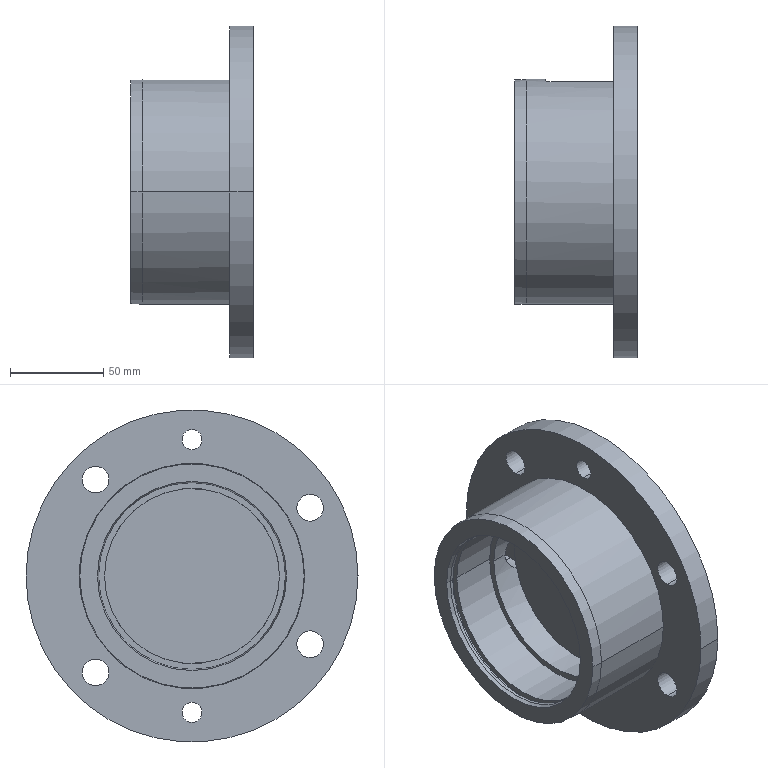Part | SolidWorks | features HoleWzd 2, ICE 2, Fillet 1, Revolution 1 | 1 solid | 44 faces | box 65.862 x 177.8 x 177.8 mm | volume 542990 mm3 | cylinder 29 | plane 11 | cone 4 | commonest cylinder face diameters 14.287 x8 10.716 x4 93.73 x4 100.013 x4 6 x2 106.02 x2
STEP:
#1=CARTESIAN_POINT('',(-18.159,45.44,-11.467));
#2=VERTEX_POINT('',#1);
#3=CARTESIAN_POINT('',(-18.159,46.865,0.));
#4=VERTEX_POINT('',#3);
#5=CARTESIAN_POINT('',(-18.159,0.,0.));
#6=DIRECTION('',(1.,0.,0.));
#7=DIRECTION('',(0.,1.,0.));
#8=AXIS2_PLACEMENT_3D('',#5,#6,#7);
#9=CIRCLE('',#8,46.865);
#10=EDGE_CURVE('',#2,#4,#9,.T.);
#11=ORIENTED_EDGE('',*,*,#10,.T.);
#12=CARTESIAN_POINT('',(-12.7,46.865,0.));
#13=VERTEX_POINT('',#12);
#14=CARTESIAN_POINT('',(0.,46.865,0.));
#15=DIRECTION('',(1.,0.,0.));
#16=VECTOR('',#15,1000.);
#17=LINE('',#14,#16);
#18=EDGE_CURVE('',#4,#13,#17,.T.);
#19=ORIENTED_EDGE('',*,*,#18,.T.);
#20=CARTESIAN_POINT('',(-12.7,45.111,-12.7));
#21=VERTEX_POINT('',#20);
#22=CARTESIAN_POINT('',(-12.7,0.,0.));
#23=DIRECTION('',(-1.,0.,0.));
#24=DIRECTION('',(0.,0.,-1.));
#25=AXIS2_PLACEMENT_3D('',#22,#23,#24);
#26=CIRCLE('',#25,46.865);
#27=EDGE_CURVE('',#13,#21,#26,.T.);
#28=ORIENTED_EDGE('',*,*,#27,.T.);
#29=CARTESIAN_POINT('',(-12.7,45.111,-12.7));
#30=CARTESIAN_POINT('',(-13.651,45.111,-12.7));
#31=CARTESIAN_POINT('',(-14.584,45.141,-12.594));
#32=CARTESIAN_POINT('',(-15.955,45.226,-12.285));
#33=CARTESIAN_POINT('',(-16.408,45.261,-12.156));
#34=CARTESIAN_POINT('',(-17.303,45.343,-11.846));
#35=CARTESIAN_POINT('',(-17.737,45.39,-11.668));
#36=CARTESIAN_POINT('',(-18.159,45.44,-11.467));
#37=B_SPLINE_CURVE_WITH_KNOTS('',3,(#29,#30,#31,#32,#33,#34,#35,#36),.UNSPECIFIED.,.F.,.F.,(4,2,2,4),(0.,0.002812,0.004219,0.005625),.UNSPECIFIED.);
#38=EDGE_CURVE('',#21,#2,#37,.T.);
#39=ORIENTED_EDGE('',*,*,#38,.T.);
#40=EDGE_LOOP('',(#11,#19,#28,#39));
#41=FACE_OUTER_BOUND('',#40,.T.);
#42=CARTESIAN_POINT('',(0.,0.,0.));
#43=DIRECTION('',(1.,0.,0.));
#44=DIRECTION('',(0.,1.,0.));
#45=AXIS2_PLACEMENT_3D('',#42,#43,#44);
#46=CYLINDRICAL_SURFACE('',#45,46.865);
#47=ADVANCED_FACE('',(#41),#46,.T.);
#48=CARTESIAN_POINT('',(-12.7,0.,67.667));
#49=VERTEX_POINT('',#48);
#50=CARTESIAN_POINT('',(-12.7,0.,78.383));
#51=VERTEX_POINT('',#50);
#52=CARTESIAN_POINT('',(-12.7,0.,73.025));
#53=DIRECTION('',(-1.,0.,0.));
#54=DIRECTION('',(0.,-1.,0.));
#55=AXIS2_PLACEMENT_3D('',#52,#53,#54);
#56=CIRCLE('',#55,5.358);
#57=EDGE_CURVE('',#49,#51,#56,.T.);
#58=ORIENTED_EDGE('',*,*,#57,.T.);
#59=CARTESIAN_POINT('',(0.,0.,78.383));
#60=VERTEX_POINT('',#59);
#61=CARTESIAN_POINT('',(0.,0.,78.383));
#62=DIRECTION('',(1.,0.,0.));
#63=VECTOR('',#62,1000.);
#64=LINE('',#61,#63);
#65=EDGE_CURVE('',#51,#60,#64,.T.);
#66=ORIENTED_EDGE('',*,*,#65,.T.);
#67=CARTESIAN_POINT('',(0.,0.,67.667));
#68=VERTEX_POINT('',#67);
#69=CARTESIAN_POINT('',(0.,0.,73.025));
#70=DIRECTION('',(1.,0.,0.));
#71=DIRECTION('',(0.,0.,-1.));
#72=AXIS2_PLACEMENT_3D('',#69,#70,#71);
#73=CIRCLE('',#72,5.358);
#74=EDGE_CURVE('',#60,#68,#73,.T.);
#75=ORIENTED_EDGE('',*,*,#74,.T.);
#76=CARTESIAN_POINT('',(0.,0.,67.667));
#77=DIRECTION('',(1.,0.,0.));
#78=VECTOR('',#77,1000.);
#79=LINE('',#76,#78);
#80=EDGE_CURVE('',#49,#68,#79,.T.);
#81=ORIENTED_EDGE('',*,*,#80,.F.);
#82=EDGE_LOOP('',(#58,#66,#75,#81));
#83=FACE_OUTER_BOUND('',#82,.T.);
#84=CARTESIAN_POINT('',(0.,0.,73.025));
#85=DIRECTION('',(1.,0.,0.));
#86=DIRECTION('',(0.,0.,-1.));
#87=AXIS2_PLACEMENT_3D('',#84,#85,#86);
#88=CYLINDRICAL_SURFACE('',#87,5.358);
#89=ADVANCED_FACE('',(#83),#88,.F.);
#90=CARTESIAN_POINT('',(-12.7,0.,-78.383));
#91=VERTEX_POINT('',#90);
#92=CARTESIAN_POINT('',(-12.7,0.,-67.667));
#93=VERTEX_POINT('',#92);
#94=CARTESIAN_POINT('',(-12.7,0.,-73.025));
#95=DIRECTION('',(-1.,0.,0.));
#96=DIRECTION('',(0.,-1.,0.));
#97=AXIS2_PLACEMENT_3D('',#94,#95,#96);
#98=CIRCLE('',#97,5.358);
#99=EDGE_CURVE('',#91,#93,#98,.T.);
#100=ORIENTED_EDGE('',*,*,#99,.T.);
#101=CARTESIAN_POINT('',(0.,0.,-67.667));
#102=VERTEX_POINT('',#101);
#103=CARTESIAN_POINT('',(0.,0.,-67.667));
#104=DIRECTION('',(1.,0.,0.));
#105=VECTOR('',#104,1000.);
#106=LINE('',#103,#105);
#107=EDGE_CURVE('',#93,#102,#106,.T.);
#108=ORIENTED_EDGE('',*,*,#107,.T.);
#109=CARTESIAN_POINT('',(0.,0.,-78.383));
#110=VERTEX_POINT('',#109);
#111=CARTESIAN_POINT('',(0.,0.,-73.025));
#112=DIRECTION('',(1.,0.,0.));
#113=DIRECTION('',(0.,0.,-1.));
#114=AXIS2_PLACEMENT_3D('',#111,#112,#113);
#115=CIRCLE('',#114,5.358);
#116=EDGE_CURVE('',#102,#110,#115,.T.);
#117=ORIENTED_EDGE('',*,*,#116,.T.);
#118=CARTESIAN_POINT('',(0.,0.,-78.383));
#119=DIRECTION('',(1.,0.,0.));
#120=VECTOR('',#119,1000.);
#121=LINE('',#118,#120);
#122=EDGE_CURVE('',#91,#110,#121,.T.);
#123=ORIENTED_EDGE('',*,*,#122,.F.);
#124=EDGE_LOOP('',(#100,#108,#117,#123));
#125=FACE_OUTER_BOUND('',#124,.T.);
#126=CARTESIAN_POINT('',(0.,0.,-73.025));
#127=DIRECTION('',(1.,0.,0.));
#128=DIRECTION('',(0.,0.,-1.));
#129=AXIS2_PLACEMENT_3D('',#126,#127,#128);
#130=CYLINDRICAL_SURFACE('',#129,5.358);
#131=ADVANCED_FACE('',(#125),#130,.F.);
#132=CARTESIAN_POINT('',(-12.7,51.638,44.494));
#133=VERTEX_POINT('',#132);
#134=CARTESIAN_POINT('',(-12.7,51.638,58.782));
#135=VERTEX_POINT('',#134);
#136=CARTESIAN_POINT('',(-12.7,51.638,51.638));
#137=DIRECTION('',(-1.,0.,0.));
#138=DIRECTION('',(0.,-1.,0.));
#139=AXIS2_PLACEMENT_3D('',#136,#137,#138);
#140=CIRCLE('',#139,7.144);
#141=EDGE_CURVE('',#133,#135,#140,.T.);
#142=ORIENTED_EDGE('',*,*,#141,.T.);
#143=CARTESIAN_POINT('',(0.,51.638,58.782));
#144=VERTEX_POINT('',#143);
#145=CARTESIAN_POINT('',(0.,51.638,58.782));
#146=DIRECTION('',(1.,0.,0.));
#147=VECTOR('',#146,1000.);
#148=LINE('',#145,#147);
#149=EDGE_CURVE('',#135,#144,#148,.T.);
#150=ORIENTED_EDGE('',*,*,#149,.T.);
#151=CARTESIAN_POINT('',(0.,51.638,44.494));
#152=VERTEX_POINT('',#151);
#153=CARTESIAN_POINT('',(0.,51.638,51.638));
#154=DIRECTION('',(1.,0.,0.));
#155=DIRECTION('',(0.,0.,-1.));
#156=AXIS2_PLACEMENT_3D('',#153,#154,#155);
#157=CIRCLE('',#156,7.144);
#158=EDGE_CURVE('',#144,#152,#157,.T.);
#159=ORIENTED_EDGE('',*,*,#158,.T.);
#160=CARTESIAN_POINT('',(0.,51.638,44.494));
#161=DIRECTION('',(1.,0.,0.));
#162=VECTOR('',#161,1000.);
#163=LINE('',#160,#162);
#164=EDGE_CURVE('',#133,#152,#163,.T.);
#165=ORIENTED_EDGE('',*,*,#164,.F.);
#166=EDGE_LOOP('',(#142,#150,#159,#165));
#167=FACE_OUTER_BOUND('',#166,.T.);
#168=CARTESIAN_POINT('',(0.,51.638,51.638));
#169=DIRECTION('',(1.,0.,0.));
#170=DIRECTION('',(0.,0.,-1.));
#171=AXIS2_PLACEMENT_3D('',#168,#169,#170);
#172=CYLINDRICAL_SURFACE('',#171,7.144);
#173=ADVANCED_FACE('',(#167),#172,.F.);
#174=CARTESIAN_POINT('',(-12.7,51.638,-58.782));
#175=VERTEX_POINT('',#174);
#176=CARTESIAN_POINT('',(-12.7,51.638,-44.494));
#177=VERTEX_POINT('',#176);
#178=CARTESIAN_POINT('',(-12.7,51.638,-51.638));
#179=DIRECTION('',(-1.,0.,0.));
#180=DIRECTION('',(0.,-1.,0.));
#181=AXIS2_PLACEMENT_3D('',#178,#179,#180);
#182=CIRCLE('',#181,7.144);
#183=EDGE_CURVE('',#175,#177,#182,.T.);
#184=ORIENTED_EDGE('',*,*,#183,.T.);
#185=CARTESIAN_POINT('',(0.,51.638,-44.494));
#186=VERTEX_POINT('',#185);
#187=CARTESIAN_POINT('',(0.,51.638,-44.494));
#188=DIRECTION('',(1.,0.,0.));
#189=VECTOR('',#188,1000.);
#190=LINE('',#187,#189);
#191=EDGE_CURVE('',#177,#186,#190,.T.);
#192=ORIENTED_EDGE('',*,*,#191,.T.);
#193=CARTESIAN_POINT('',(0.,51.638,-58.782));
#194=VERTEX_POINT('',#193);
#195=CARTESIAN_POINT('',(0.,51.638,-51.638));
#196=DIRECTION('',(1.,0.,0.));
#197=DIRECTION('',(0.,0.,-1.));
#198=AXIS2_PLACEMENT_3D('',#195,#196,#197);
#199=CIRCLE('',#198,7.144);
#200=EDGE_CURVE('',#186,#194,#199,.T.);
#201=ORIENTED_EDGE('',*,*,#200,.T.);
#202=CARTESIAN_POINT('',(0.,51.638,-58.782));
#203=DIRECTION('',(1.,0.,0.));
#204=VECTOR('',#203,1000.);
#205=LINE('',#202,#204);
#206=EDGE_CURVE('',#175,#194,#205,.T.);
#207=ORIENTED_EDGE('',*,*,#206,.F.);
#208=EDGE_LOOP('',(#184,#192,#201,#207));
#209=FACE_OUTER_BOUND('',#208,.T.);
#210=CARTESIAN_POINT('',(0.,51.638,-51.638));
#211=DIRECTION('',(1.,0.,0.));
#212=DIRECTION('',(0.,0.,-1.));
#213=AXIS2_PLACEMENT_3D('',#210,#211,#212);
#214=CYLINDRICAL_SURFACE('',#213,7.144);
#215=ADVANCED_FACE('',(#209),#214,.F.);
#216=CARTESIAN_POINT('',(-12.7,-63.246,29.381));
#217=VERTEX_POINT('',#216);
#218=CARTESIAN_POINT('',(-12.7,-63.246,43.669));
#219=VERTEX_POINT('',#218);
#220=CARTESIAN_POINT('',(-12.7,-63.246,36.525));
#221=DIRECTION('',(-1.,0.,0.));
#222=DIRECTION('',(0.,-1.,0.));
#223=AXIS2_PLACEMENT_3D('',#220,#221,#222);
#224=CIRCLE('',#223,7.144);
#225=EDGE_CURVE('',#217,#219,#224,.T.);
#226=ORIENTED_EDGE('',*,*,#225,.T.);
#227=CARTESIAN_POINT('',(0.,-63.246,43.669));
#228=VERTEX_POINT('',#227);
#229=CARTESIAN_POINT('',(0.,-63.246,43.669));
#230=DIRECTION('',(1.,0.,0.));
#231=VECTOR('',#230,1000.);
#232=LINE('',#229,#231);
#233=EDGE_CURVE('',#219,#228,#232,.T.);
#234=ORIENTED_EDGE('',*,*,#233,.T.);
#235=CARTESIAN_POINT('',(0.,-63.246,29.381));
#236=VERTEX_POINT('',#235);
#237=CARTESIAN_POINT('',(0.,-63.246,36.525));
#238=DIRECTION('',(1.,0.,0.));
#239=DIRECTION('',(0.,0.,-1.));
#240=AXIS2_PLACEMENT_3D('',#237,#238,#239);
#241=CIRCLE('',#240,7.144);
#242=EDGE_CURVE('',#228,#236,#241,.T.);
#243=ORIENTED_EDGE('',*,*,#242,.T.);
#244=CARTESIAN_POINT('',(0.,-63.246,29.381));
#245=DIRECTION('',(1.,0.,0.));
#246=VECTOR('',#245,1000.);
#247=LINE('',#244,#246);
#248=EDGE_CURVE('',#217,#236,#247,.T.);
#249=ORIENTED_EDGE('',*,*,#248,.F.);
#250=EDGE_LOOP('',(#226,#234,#243,#249));
#251=FACE_OUTER_BOUND('',#250,.T.);
#252=CARTESIAN_POINT('',(0.,-63.246,36.525));
#253=DIRECTION('',(1.,0.,0.));
#254=DIRECTION('',(0.,0.,-1.));
#255=AXIS2_PLACEMENT_3D('',#252,#253,#254);
#256=CYLINDRICAL_SURFACE('',#255,7.144);
#257=ADVANCED_FACE('',(#251),#256,.F.);
#258=CARTESIAN_POINT('',(-12.7,-63.246,-43.669));
#259=VERTEX_POINT('',#258);
#260=CARTESIAN_POINT('',(-12.7,-63.246,-29.381));
#261=VERTEX_POINT('',#260);
#262=CARTESIAN_POINT('',(-12.7,-63.246,-36.525));
#263=DIRECTION('',(-1.,0.,0.));
#264=DIRECTION('',(0.,-1.,0.));
#265=AXIS2_PLACEMENT_3D('',#262,#263,#264);
#266=CIRCLE('',#265,7.144);
#267=EDGE_CURVE('',#259,#261,#266,.T.);
#268=ORIENTED_EDGE('',*,*,#267,.T.);
#269=CARTESIAN_POINT('',(0.,-63.246,-29.381));
#270=VERTEX_POINT('',#269);
#271=CARTESIAN_POINT('',(0.,-63.246,-29.381));
#272=DIRECTION('',(1.,0.,0.));
#273=VECTOR('',#272,1000.);
#274=LINE('',#271,#273);
#275=EDGE_CURVE('',#261,#270,#274,.T.);
#276=ORIENTED_EDGE('',*,*,#275,.T.);
#277=CARTESIAN_POINT('',(0.,-63.246,-43.669));
#278=VERTEX_POINT('',#277);
#279=CARTESIAN_POINT('',(0.,-63.246,-36.525));
#280=DIRECTION('',(1.,0.,0.));
#281=DIRECTION('',(0.,0.,-1.));
#282=AXIS2_PLACEMENT_3D('',#279,#280,#281);
#283=CIRCLE('',#282,7.144);
#284=EDGE_CURVE('',#270,#278,#283,.T.);
#285=ORIENTED_EDGE('',*,*,#284,.T.);
#286=CARTESIAN_POINT('',(0.,-63.246,-43.669));
#287=DIRECTION('',(1.,0.,0.));
#288=VECTOR('',#287,1000.);
#289=LINE('',#286,#288);
#290=EDGE_CURVE('',#259,#278,#289,.T.);
#291=ORIENTED_EDGE('',*,*,#290,.F.);
#292=EDGE_LOOP('',(#268,#276,#285,#291));
#293=FACE_OUTER_BOUND('',#292,.T.);
#294=CARTESIAN_POINT('',(0.,-63.246,-36.525));
#295=DIRECTION('',(1.,0.,0.));
#296=DIRECTION('',(0.,0.,-1.));
#297=AXIS2_PLACEMENT_3D('',#294,#295,#296);
#298=CYLINDRICAL_SURFACE('',#297,7.144);
#299=ADVANCED_FACE('',(#293),#298,.F.);
#300=CARTESIAN_POINT('',(-12.7,88.9,0.));
#301=VERTEX_POINT('',#300);
#302=CARTESIAN_POINT('',(-12.7,-88.9,0.));
#303=VERTEX_POINT('',#302);
#304=CARTESIAN_POINT('',(-12.7,0.,0.));
#305=DIRECTION('',(1.,0.,0.));
#306=DIRECTION('',(0.,1.,0.));
#307=AXIS2_PLACEMENT_3D('',#304,#305,#306);
#308=CIRCLE('',#307,88.9);
#309=EDGE_CURVE('',#301,#303,#308,.T.);
#310=ORIENTED_EDGE('',*,*,#309,.T.);
#311=CARTESIAN_POINT('',(0.,-88.9,0.));
#312=VERTEX_POINT('',#311);
#313=CARTESIAN_POINT('',(0.,-88.9,0.));
#314=DIRECTION('',(1.,0.,0.));
#315=VECTOR('',#314,1000.);
#316=LINE('',#313,#315);
#317=EDGE_CURVE('',#303,#312,#316,.T.);
#318=ORIENTED_EDGE('',*,*,#317,.T.);
#319=CARTESIAN_POINT('',(0.,88.9,0.));
#320=VERTEX_POINT('',#319);
#321=CARTESIAN_POINT('',(0.,0.,0.));
#322=DIRECTION('',(1.,0.,0.));
#323=DIRECTION('',(0.,1.,0.));
#324=AXIS2_PLACEMENT_3D('',#321,#322,#323);
#325=CIRCLE('',#324,88.9);
#326=EDGE_CURVE('',#320,#312,#325,.T.);
#327=ORIENTED_EDGE('',*,*,#326,.F.);
#328=CARTESIAN_POINT('',(0.,88.9,0.));
#329=DIRECTION('',(1.,0.,0.));
#330=VECTOR('',#329,1000.);
#331=LINE('',#328,#330);
#332=EDGE_CURVE('',#301,#320,#331,.T.);
#333=ORIENTED_EDGE('',*,*,#332,.F.);
#334=EDGE_LOOP('',(#310,#318,#327,#333));
#335=FACE_OUTER_BOUND('',#334,.T.);
#336=CARTESIAN_POINT('',(0.,0.,0.));
#337=DIRECTION('',(1.,0.,0.));
#338=DIRECTION('',(0.,1.,0.));
#339=AXIS2_PLACEMENT_3D('',#336,#337,#338);
#340=CYLINDRICAL_SURFACE('',#339,88.9);
#341=ADVANCED_FACE('',(#335),#340,.T.);
#342=CARTESIAN_POINT('',(-59.512,60.312,0.));
#343=VERTEX_POINT('',#342);
#344=CARTESIAN_POINT('',(-59.512,-60.312,0.));
#345=VERTEX_POINT('',#344);
#346=CARTESIAN_POINT('',(-59.512,0.,0.));
#347=DIRECTION('',(1.,0.,0.));
#348=DIRECTION('',(0.,1.,0.));
#349=AXIS2_PLACEMENT_3D('',#346,#347,#348);
#350=CIRCLE('',#349,60.312);
#351=EDGE_CURVE('',#343,#345,#350,.T.);
#352=ORIENTED_EDGE('',*,*,#351,.T.);
#353=CARTESIAN_POINT('',(-12.7,-60.312,0.));
#354=VERTEX_POINT('',#353);
#355=CARTESIAN_POINT('',(0.,-60.312,0.));
#356=DIRECTION('',(1.,0.,0.));
#357=VECTOR('',#356,1000.);
#358=LINE('',#355,#357);
#359=EDGE_CURVE('',#345,#354,#358,.T.);
#360=ORIENTED_EDGE('',*,*,#359,.T.);
#361=CARTESIAN_POINT('',(-12.7,58.96,12.7));
#362=VERTEX_POINT('',#361);
#363=CARTESIAN_POINT('',(-12.7,0.,0.));
#364=DIRECTION('',(1.,0.,0.));
#365=DIRECTION('',(0.,1.,0.));
#366=AXIS2_PLACEMENT_3D('',#363,#364,#365);
#367=CIRCLE('',#366,60.312);
#368=EDGE_CURVE('',#362,#354,#367,.T.);
#369=ORIENTED_EDGE('',*,*,#368,.F.);
#370=CARTESIAN_POINT('',(-46.276,58.96,12.7));
#371=VERTEX_POINT('',#370);
#372=CARTESIAN_POINT('',(0.,58.96,12.7));
#373=DIRECTION('',(1.,0.,0.));
#374=VECTOR('',#373,1000.);
#375=LINE('',#372,#374);
#376=EDGE_CURVE('',#371,#362,#375,.T.);
#377=ORIENTED_EDGE('',*,*,#376,.F.);
#378=CARTESIAN_POINT('',(-49.276,59.527,9.7));
#379=VERTEX_POINT('',#378);
#380=CARTESIAN_POINT('',(-46.276,58.96,12.7));
#381=CARTESIAN_POINT('',(-46.476,58.96,12.7));
#382=CARTESIAN_POINT('',(-46.672,58.964,12.68));
#383=CARTESIAN_POINT('',(-47.058,58.981,12.603));
#384=CARTESIAN_POINT('',(-47.25,58.993,12.544));
#385=CARTESIAN_POINT('',(-47.614,59.026,12.392));
#386=CARTESIAN_POINT('',(-47.787,59.045,12.299));
#387=CARTESIAN_POINT('',(-48.113,59.09,12.08));
#388=CARTESIAN_POINT('',(-48.267,59.116,11.953));
#389=CARTESIAN_POINT('',(-48.68,59.199,11.537));
#390=CARTESIAN_POINT('',(-48.901,59.264,11.204));
#391=CARTESIAN_POINT('',(-49.123,59.362,10.665));
#392=CARTESIAN_POINT('',(-49.18,59.396,10.476));
#393=CARTESIAN_POINT('',(-49.257,59.462,10.092));
#394=CARTESIAN_POINT('',(-49.276,59.495,9.897));
#395=CARTESIAN_POINT('',(-49.276,59.527,9.7));
#396=B_SPLINE_CURVE_WITH_KNOTS('',3,(#380,#381,#382,#383,#384,#385,#386,#387,#388,#389,#390,#391,#392,#393,#394,#395),.UNSPECIFIED.,.F.,.F.,(4,2,2,2,2,2,2,4),(0.,0.0005908,0.001182,0.001772,0.002363,0.003545,0.004136,0.004727),.UNSPECIFIED.);
#397=EDGE_CURVE('',#371,#379,#396,.T.);
#398=ORIENTED_EDGE('',*,*,#397,.T.);
#399=CARTESIAN_POINT('',(-49.276,60.312,0.));
#400=VERTEX_POINT('',#399);
#401=CARTESIAN_POINT('',(-49.276,0.,0.));
#402=DIRECTION('',(1.,0.,0.));
#403=DIRECTION('',(0.,0.,1.));
#404=AXIS2_PLACEMENT_3D('',#401,#402,#403);
#405=CIRCLE('',#404,60.312);
#406=EDGE_CURVE('',#400,#379,#405,.T.);
#407=ORIENTED_EDGE('',*,*,#406,.F.);
#408=CARTESIAN_POINT('',(0.,60.312,0.));
#409=DIRECTION('',(1.,0.,0.));
#410=VECTOR('',#409,1000.);
#411=LINE('',#408,#410);
#412=EDGE_CURVE('',#343,#400,#411,.T.);
#413=ORIENTED_EDGE('',*,*,#412,.F.);
#414=EDGE_LOOP('',(#352,#360,#369,#377,#398,#407,#413));
#415=FACE_OUTER_BOUND('',#414,.T.);
#416=CARTESIAN_POINT('',(0.,0.,0.));
#417=DIRECTION('',(1.,0.,0.));
#418=DIRECTION('',(0.,1.,0.));
#419=AXIS2_PLACEMENT_3D('',#416,#417,#418);
#420=CYLINDRICAL_SURFACE('',#419,60.312);
#421=ADVANCED_FACE('',(#415),#420,.T.);
#422=CARTESIAN_POINT('',(-65.862,60.07,0.));
#423=VERTEX_POINT('',#422);
#424=CARTESIAN_POINT('',(-65.862,-60.071,0.));
#425=VERTEX_POINT('',#424);
#426=CARTESIAN_POINT('',(-65.862,0.,0.));
#427=DIRECTION('',(1.,0.,0.));
#428=DIRECTION('',(0.,1.,0.));
#429=AXIS2_PLACEMENT_3D('',#426,#427,#428);
#430=CIRCLE('',#429,60.071);
#431=EDGE_CURVE('',#423,#425,#430,.T.);
#432=ORIENTED_EDGE('',*,*,#431,.T.);
#433=CARTESIAN_POINT('',(-59.512,-60.312,0.));
#434=DIRECTION('',(0.9993,-0.03805,0.));
#435=VECTOR('',#434,1000.);
#436=LINE('',#433,#435);
#437=EDGE_CURVE('',#425,#345,#436,.T.);
#438=ORIENTED_EDGE('',*,*,#437,.T.);
#439=ORIENTED_EDGE('',*,*,#351,.F.);
#440=CARTESIAN_POINT('',(-59.512,60.312,0.));
#441=DIRECTION('',(0.9993,0.03805,0.));
#442=VECTOR('',#441,1000.);
#443=LINE('',#440,#442);
#444=EDGE_CURVE('',#423,#343,#443,.T.);
#445=ORIENTED_EDGE('',*,*,#444,.F.);
#446=EDGE_LOOP('',(#432,#438,#439,#445));
#447=FACE_OUTER_BOUND('',#446,.T.);
#448=CARTESIAN_POINT('',(-59.512,0.,0.));
#449=DIRECTION('',(1.,0.,0.));
#450=DIRECTION('',(0.,1.,0.));
#451=AXIS2_PLACEMENT_3D('',#448,#449,#450);
#452=CONICAL_SURFACE('',#451,60.312,0.03806);
#453=ADVANCED_FACE('',(#447),#452,.T.);
#454=CARTESIAN_POINT('',(-63.576,-50.006,0.));
#455=VERTEX_POINT('',#454);
#456=CARTESIAN_POINT('',(-63.576,50.006,0.));
#457=VERTEX_POINT('',#456);
#458=CARTESIAN_POINT('',(-63.576,0.,0.));
#459=DIRECTION('',(1.,0.,0.));
#460=DIRECTION('',(0.,1.,0.));
#461=AXIS2_PLACEMENT_3D('',#458,#459,#460);
#462=CIRCLE('',#461,50.006);
#463=EDGE_CURVE('',#455,#457,#462,.T.);
#464=ORIENTED_EDGE('',*,*,#463,.T.);
#465=CARTESIAN_POINT('',(-65.862,50.619,0.));
#466=VERTEX_POINT('',#465);
#467=CARTESIAN_POINT('',(-65.862,50.619,0.));
#468=DIRECTION('',(-0.9659,0.2588,0.));
#469=VECTOR('',#468,1000.);
#470=LINE('',#467,#469);
#471=EDGE_CURVE('',#457,#466,#470,.T.);
#472=ORIENTED_EDGE('',*,*,#471,.T.);
#473=CARTESIAN_POINT('',(-65.862,-50.619,0.));
#474=VERTEX_POINT('',#473);
#475=CARTESIAN_POINT('',(-65.862,0.,0.));
#476=DIRECTION('',(1.,0.,0.));
#477=DIRECTION('',(0.,1.,0.));
#478=AXIS2_PLACEMENT_3D('',#475,#476,#477);
#479=CIRCLE('',#478,50.619);
#480=EDGE_CURVE('',#474,#466,#479,.T.);
#481=ORIENTED_EDGE('',*,*,#480,.F.);
#482=CARTESIAN_POINT('',(-65.862,-50.619,0.));
#483=DIRECTION('',(-0.9659,-0.2588,0.));
#484=VECTOR('',#483,1000.);
#485=LINE('',#482,#484);
#486=EDGE_CURVE('',#455,#474,#485,.T.);
#487=ORIENTED_EDGE('',*,*,#486,.F.);
#488=EDGE_LOOP('',(#464,#472,#481,#487));
#489=FACE_OUTER_BOUND('',#488,.T.);
#490=CARTESIAN_POINT('',(-65.862,0.,0.));
#491=DIRECTION('',(-1.,0.,0.));
#492=DIRECTION('',(0.,-1.,0.));
#493=AXIS2_PLACEMENT_3D('',#490,#491,#492);
#494=CONICAL_SURFACE('',#493,50.619,0.2618);
#495=ADVANCED_FACE('',(#489),#494,.F.);
#496=ORIENTED_EDGE('',*,*,#463,.F.);
#497=CARTESIAN_POINT('',(-61.824,-50.006,0.));
#498=VERTEX_POINT('',#497);
#499=CARTESIAN_POINT('',(0.,-50.006,0.));
#500=DIRECTION('',(1.,0.,0.));
#501=VECTOR('',#500,1000.);
#502=LINE('',#499,#501);
#503=EDGE_CURVE('',#455,#498,#502,.T.);
#504=ORIENTED_EDGE('',*,*,#503,.T.);
#505=CARTESIAN_POINT('',(-61.824,50.006,0.));
#506=VERTEX_POINT('',#505);
#507=CARTESIAN_POINT('',(-61.824,0.,0.));
#508=DIRECTION('',(1.,0.,0.));
#509=DIRECTION('',(0.,1.,0.));
#510=AXIS2_PLACEMENT_3D('',#507,#508,#509);
#511=CIRCLE('',#510,50.006);
#512=EDGE_CURVE('',#498,#506,#511,.T.);
#513=ORIENTED_EDGE('',*,*,#512,.T.);
#514=CARTESIAN_POINT('',(0.,50.006,0.));
#515=DIRECTION('',(1.,0.,0.));
#516=VECTOR('',#515,1000.);
#517=LINE('',#514,#516);
#518=EDGE_CURVE('',#457,#506,#517,.T.);
#519=ORIENTED_EDGE('',*,*,#518,.F.);
#520=EDGE_LOOP('',(#496,#504,#513,#519));
#521=FACE_OUTER_BOUND('',#520,.T.);
#522=CARTESIAN_POINT('',(0.,0.,0.));
#523=DIRECTION('',(1.,0.,0.));
#524=DIRECTION('',(0.,1.,0.));
#525=AXIS2_PLACEMENT_3D('',#522,#523,#524);
#526=CYLINDRICAL_SURFACE('',#525,50.006);
#527=ADVANCED_FACE('',(#521),#526,.F.);
#528=CARTESIAN_POINT('',(-61.824,-53.01,0.));
#529=VERTEX_POINT('',#528);
#530=CARTESIAN_POINT('',(-61.824,53.01,0.));
#531=VERTEX_POINT('',#530);
#532=CARTESIAN_POINT('',(-61.824,0.,0.));
#533=DIRECTION('',(1.,0.,0.));
#534=DIRECTION('',(0.,1.,0.));
#535=AXIS2_PLACEMENT_3D('',#532,#533,#534);
#536=CIRCLE('',#535,53.01);
#537=EDGE_CURVE('',#529,#531,#536,.T.);
#538=ORIENTED_EDGE('',*,*,#537,.F.);
#539=CARTESIAN_POINT('',(-58.776,-53.01,0.));
#540=VERTEX_POINT('',#539);
#541=CARTESIAN_POINT('',(0.,-53.01,0.));
#542=DIRECTION('',(1.,0.,0.));
#543=VECTOR('',#542,1000.);
#544=LINE('',#541,#543);
#545=EDGE_CURVE('',#529,#540,#544,.T.);
#546=ORIENTED_EDGE('',*,*,#545,.T.);
#547=CARTESIAN_POINT('',(-58.776,53.01,0.));
#548=VERTEX_POINT('',#547);
#549=CARTESIAN_POINT('',(-58.776,0.,0.));
#550=DIRECTION('',(1.,0.,0.));
#551=DIRECTION('',(0.,1.,0.));
#552=AXIS2_PLACEMENT_3D('',#549,#550,#551);
#553=CIRCLE('',#552,53.01);
#554=EDGE_CURVE('',#540,#548,#553,.T.);
#555=ORIENTED_EDGE('',*,*,#554,.T.);
#556=CARTESIAN_POINT('',(0.,53.01,0.));
#557=DIRECTION('',(1.,0.,0.));
#558=VECTOR('',#557,1000.);
#559=LINE('',#556,#558);
#560=EDGE_CURVE('',#531,#548,#559,.T.);
#561=ORIENTED_EDGE('',*,*,#560,.F.);
#562=EDGE_LOOP('',(#538,#546,#555,#561));
#563=FACE_OUTER_BOUND('',#562,.T.);
#564=CARTESIAN_POINT('',(0.,0.,0.));
#565=DIRECTION('',(1.,0.,0.));
#566=DIRECTION('',(0.,1.,0.));
#567=AXIS2_PLACEMENT_3D('',#564,#565,#566);
#568=CYLINDRICAL_SURFACE('',#567,53.01);
#569=ADVANCED_FACE('',(#563),#568,.F.);
#570=CARTESIAN_POINT('',(-58.776,-50.006,0.));
#571=VERTEX_POINT('',#570);
#572=CARTESIAN_POINT('',(-58.776,50.006,0.));
#573=VERTEX_POINT('',#572);
#574=CARTESIAN_POINT('',(-58.776,0.,0.));
#575=DIRECTION('',(1.,0.,0.));
#576=DIRECTION('',(0.,1.,0.));
#577=AXIS2_PLACEMENT_3D('',#574,#575,#576);
#578=CIRCLE('',#577,50.006);
#579=EDGE_CURVE('',#571,#573,#578,.T.);
#580=ORIENTED_EDGE('',*,*,#579,.F.);
#581=CARTESIAN_POINT('',(-33.909,-50.006,0.));
#582=VERTEX_POINT('',#581);
#583=CARTESIAN_POINT('',(0.,-50.006,0.));
#584=DIRECTION('',(1.,0.,0.));
#585=VECTOR('',#584,1000.);
#586=LINE('',#583,#585);
#587=EDGE_CURVE('',#571,#582,#586,.T.);
#588=ORIENTED_EDGE('',*,*,#587,.T.);
#589=CARTESIAN_POINT('',(-33.909,50.006,0.));
#590=VERTEX_POINT('',#589);
#591=CARTESIAN_POINT('',(-33.909,0.,0.));
#592=DIRECTION('',(1.,0.,0.));
#593=DIRECTION('',(0.,1.,0.));
#594=AXIS2_PLACEMENT_3D('',#591,#592,#593);
#595=CIRCLE('',#594,50.006);
#596=EDGE_CURVE('',#582,#590,#595,.T.);
#597=ORIENTED_EDGE('',*,*,#596,.T.);
#598=CARTESIAN_POINT('',(0.,50.006,0.));
#599=DIRECTION('',(1.,0.,0.));
#600=VECTOR('',#599,1000.);
#601=LINE('',#598,#600);
#602=EDGE_CURVE('',#573,#590,#601,.T.);
#603=ORIENTED_EDGE('',*,*,#602,.F.);
#604=EDGE_LOOP('',(#580,#588,#597,#603));
#605=FACE_OUTER_BOUND('',#604,.T.);
#606=CARTESIAN_POINT('',(0.,0.,0.));
#607=DIRECTION('',(1.,0.,0.));
#608=DIRECTION('',(0.,1.,0.));
#609=AXIS2_PLACEMENT_3D('',#606,#607,#608);
#610=CYLINDRICAL_SURFACE('',#609,50.006);
#611=ADVANCED_FACE('',(#605),#610,.F.);
#612=CARTESIAN_POINT('',(-33.909,-46.865,0.));
#613=VERTEX_POINT('',#612);
#614=CARTESIAN_POINT('',(-33.909,46.865,0.));
#615=VERTEX_POINT('',#614);
#616=CARTESIAN_POINT('',(-33.909,0.,0.));
#617=DIRECTION('',(1.,0.,0.));
#618=DIRECTION('',(0.,1.,0.));
#619=AXIS2_PLACEMENT_3D('',#616,#617,#618);
#620=CIRCLE('',#619,46.865);
#621=EDGE_CURVE('',#613,#615,#620,.T.);
#622=ORIENTED_EDGE('',*,*,#621,.F.);
#623=CARTESIAN_POINT('',(-18.159,-46.865,0.));
#624=VERTEX_POINT('',#623);
#625=CARTESIAN_POINT('',(0.,-46.865,0.));
#626=DIRECTION('',(1.,0.,0.));
#627=VECTOR('',#626,1000.);
#628=LINE('',#625,#627);
#629=EDGE_CURVE('',#613,#624,#628,.T.);
#630=ORIENTED_EDGE('',*,*,#629,.T.);
#631=CARTESIAN_POINT('',(-18.159,0.,0.));
#632=DIRECTION('',(1.,0.,0.));
#633=DIRECTION('',(0.,1.,0.));
#634=AXIS2_PLACEMENT_3D('',#631,#632,#633);
#635=CIRCLE('',#634,46.865);
#636=EDGE_CURVE('',#624,#2,#635,.T.);
#637=ORIENTED_EDGE('',*,*,#636,.T.);
#638=CARTESIAN_POINT('',(-25.4,46.865,0.));
#639=VERTEX_POINT('',#638);
#640=CARTESIAN_POINT('',(-18.159,45.44,-11.467));
#641=CARTESIAN_POINT('',(-18.696,45.505,-11.211));
#642=CARTESIAN_POINT('',(-19.212,45.576,-10.919));
#643=CARTESIAN_POINT('',(-20.205,45.729,-10.263));
#644=CARTESIAN_POINT('',(-20.683,45.81,-9.895));
#645=CARTESIAN_POINT('',(-21.573,45.974,-9.106));
#646=CARTESIAN_POINT('',(-21.987,46.056,-8.683));
#647=CARTESIAN_POINT('',(-22.754,46.217,-7.781));
#648=CARTESIAN_POINT('',(-23.109,46.296,-7.3));
#649=CARTESIAN_POINT('',(-24.072,46.518,-5.781));
#650=CARTESIAN_POINT('',(-24.56,46.643,-4.699));
#651=CARTESIAN_POINT('',(-24.978,46.752,-3.259));
#652=CARTESIAN_POINT('',(-25.053,46.772,-2.965));
#653=CARTESIAN_POINT('',(-25.179,46.806,-2.377));
#654=CARTESIAN_POINT('',(-25.232,46.82,-2.081));
#655=CARTESIAN_POINT('',(-25.358,46.854,-1.193));
#656=CARTESIAN_POINT('',(-25.4,46.865,-0.5982));
#657=CARTESIAN_POINT('',(-25.4,46.865,0.));
#658=B_SPLINE_CURVE_WITH_KNOTS('',3,(#640,#641,#642,#643,#644,#645,#646,#647,#648,#649,#650,#651,#652,#653,#654,#655,#656,#657),.UNSPECIFIED.,.F.,.F.,(4,2,2,2,2,2,2,2,4),(0.005625,0.007416,0.009207,0.011,0.01279,0.01637,0.01727,0.01816,0.01995),.UNSPECIFIED.);
#659=EDGE_CURVE('',#2,#639,#658,.T.);
#660=ORIENTED_EDGE('',*,*,#659,.T.);
#661=CARTESIAN_POINT('',(0.,46.865,0.));
#662=DIRECTION('',(1.,0.,0.));
#663=VECTOR('',#662,1000.);
#664=LINE('',#661,#663);
#665=EDGE_CURVE('',#615,#639,#664,.T.);
#666=ORIENTED_EDGE('',*,*,#665,.F.);
#667=EDGE_LOOP('',(#622,#630,#637,#660,#666));
#668=FACE_OUTER_BOUND('',#667,.T.);
#669=CARTESIAN_POINT('',(0.,0.,0.));
#670=DIRECTION('',(1.,0.,0.));
#671=DIRECTION('',(0.,1.,0.));
#672=AXIS2_PLACEMENT_3D('',#669,#670,#671);
#673=CYLINDRICAL_SURFACE('',#672,46.865);
#674=ADVANCED_FACE('',(#668),#673,.F.);
#675=CARTESIAN_POINT('',(-18.159,45.44,11.467));
#676=VERTEX_POINT('',#675);
#677=CARTESIAN_POINT('',(-18.159,0.,0.));
#678=DIRECTION('',(1.,0.,0.));
#679=DIRECTION('',(0.,1.,0.));
#680=AXIS2_PLACEMENT_3D('',#677,#678,#679);
#681=CIRCLE('',#680,46.865);
#682=EDGE_CURVE('',#676,#624,#681,.T.);
#683=ORIENTED_EDGE('',*,*,#682,.F.);
#684=CARTESIAN_POINT('',(-18.159,0.,0.));
#685=DIRECTION('',(1.,0.,0.));
#686=DIRECTION('',(0.,1.,0.));
#687=AXIS2_PLACEMENT_3D('',#684,#685,#686);
#688=CIRCLE('',#687,46.865);
#689=EDGE_CURVE('',#4,#676,#688,.T.);
#690=ORIENTED_EDGE('',*,*,#689,.F.);
#691=ORIENTED_EDGE('',*,*,#10,.F.);
#692=ORIENTED_EDGE('',*,*,#636,.F.);
#693=EDGE_LOOP('',(#683,#690,#691,#692));
#694=FACE_OUTER_BOUND('',#693,.T.);
#695=CARTESIAN_POINT('',(-18.159,0.,0.));
#696=DIRECTION('',(-1.,0.,0.));
#697=DIRECTION('',(0.,-1.,0.));
#698=AXIS2_PLACEMENT_3D('',#695,#696,#697);
#699=PLANE('',#698);
#700=ADVANCED_FACE('',(#694),#699,.T.);
#701=ORIENTED_EDGE('',*,*,#629,.F.);
#702=CARTESIAN_POINT('',(-33.909,0.,0.));
#703=DIRECTION('',(1.,0.,0.));
#704=DIRECTION('',(0.,1.,0.));
#705=AXIS2_PLACEMENT_3D('',#702,#703,#704);
#706=CIRCLE('',#705,46.865);
#707=EDGE_CURVE('',#615,#613,#706,.T.);
#708=ORIENTED_EDGE('',*,*,#707,.F.);
#709=ORIENTED_EDGE('',*,*,#665,.T.);
#710=CARTESIAN_POINT('',(-25.4,46.865,0.));
#711=CARTESIAN_POINT('',(-25.4,46.865,0.2987));
#712=CARTESIAN_POINT('',(-25.389,46.862,0.5983));
#713=CARTESIAN_POINT('',(-25.347,46.851,1.199));
#714=CARTESIAN_POINT('',(-25.315,46.842,1.5));
#715=CARTESIAN_POINT('',(-25.187,46.808,2.392));
#716=CARTESIAN_POINT('',(-25.061,46.774,2.975));
#717=CARTESIAN_POINT('',(-24.729,46.687,4.118));
#718=CARTESIAN_POINT('',(-24.522,46.634,4.678));
#719=CARTESIAN_POINT('',(-24.027,46.511,5.775));
#720=CARTESIAN_POINT('',(-23.744,46.443,6.299));
#721=CARTESIAN_POINT('',(-23.11,46.296,7.299));
#722=CARTESIAN_POINT('',(-22.759,46.218,7.776));
#723=CARTESIAN_POINT('',(-22.18,46.096,8.456));
#724=CARTESIAN_POINT('',(-21.977,46.055,8.678));
#725=CARTESIAN_POINT('',(-21.56,45.973,9.104));
#726=CARTESIAN_POINT('',(-21.344,45.932,9.309));
#727=CARTESIAN_POINT('',(-20.679,45.81,9.898));
#728=CARTESIAN_POINT('',(-20.211,45.73,10.258));
#729=CARTESIAN_POINT('',(-19.47,45.616,10.749));
#730=CARTESIAN_POINT('',(-19.216,45.579,10.905));
#731=CARTESIAN_POINT('',(-18.696,45.507,11.199));
#732=CARTESIAN_POINT('',(-18.429,45.473,11.338));
#733=CARTESIAN_POINT('',(-18.159,45.44,11.467));
#734=B_SPLINE_CURVE_WITH_KNOTS('',3,(#710,#711,#712,#713,#714,#715,#716,#717,#718,#719,#720,#721,#722,#723,#724,#725,#726,#727,#728,#729,#730,#731,#732,#733),.UNSPECIFIED.,.F.,.F.,(4,2,2,2,2,2,2,2,2,2,2,4),(0.01995,0.02085,0.02174,0.02353,0.02532,0.02711,0.0289,0.02979,0.03068,0.03247,0.03337,0.03426),.UNSPECIFIED.);
#735=EDGE_CURVE('',#639,#676,#734,.T.);
#736=ORIENTED_EDGE('',*,*,#735,.T.);
#737=ORIENTED_EDGE('',*,*,#682,.T.);
#738=EDGE_LOOP('',(#701,#708,#709,#736,#737));
#739=FACE_OUTER_BOUND('',#738,.T.);
#740=CARTESIAN_POINT('',(0.,0.,0.));
#741=DIRECTION('',(1.,0.,0.));
#742=DIRECTION('',(0.,1.,0.));
#743=AXIS2_PLACEMENT_3D('',#740,#741,#742);
#744=CYLINDRICAL_SURFACE('',#743,46.865);
#745=ADVANCED_FACE('',(#739),#744,.F.);
#746=ORIENTED_EDGE('',*,*,#707,.T.);
#747=ORIENTED_EDGE('',*,*,#621,.T.);
#748=EDGE_LOOP('',(#746,#747));
#749=FACE_BOUND('',#748,.T.);
#750=CARTESIAN_POINT('',(-33.909,0.,0.));
#751=DIRECTION('',(1.,0.,0.));
#752=DIRECTION('',(0.,1.,0.));
#753=AXIS2_PLACEMENT_3D('',#750,#751,#752);
#754=CIRCLE('',#753,50.006);
#755=EDGE_CURVE('',#590,#582,#754,.T.);
#756=ORIENTED_EDGE('',*,*,#755,.F.);
#757=ORIENTED_EDGE('',*,*,#596,.F.);
#758=EDGE_LOOP('',(#756,#757));
#759=FACE_OUTER_BOUND('',#758,.T.);
#760=CARTESIAN_POINT('',(-33.909,46.865,0.));
#761=DIRECTION('',(-1.,0.,0.));
#762=DIRECTION('',(0.,-1.,0.));
#763=AXIS2_PLACEMENT_3D('',#760,#761,#762);
#764=PLANE('',#763);
#765=ADVANCED_FACE('',(#749,#759),#764,.T.);
#766=ORIENTED_EDGE('',*,*,#587,.F.);
#767=CARTESIAN_POINT('',(-58.776,0.,0.));
#768=DIRECTION('',(1.,0.,0.));
#769=DIRECTION('',(0.,1.,0.));
#770=AXIS2_PLACEMENT_3D('',#767,#768,#769);
#771=CIRCLE('',#770,50.006);
#772=EDGE_CURVE('',#573,#571,#771,.T.);
#773=ORIENTED_EDGE('',*,*,#772,.F.);
#774=ORIENTED_EDGE('',*,*,#602,.T.);
#775=ORIENTED_EDGE('',*,*,#755,.T.);
#776=EDGE_LOOP('',(#766,#773,#774,#775));
#777=FACE_OUTER_BOUND('',#776,.T.);
#778=CARTESIAN_POINT('',(0.,0.,0.));
#779=DIRECTION('',(1.,0.,0.));
#780=DIRECTION('',(0.,1.,0.));
#781=AXIS2_PLACEMENT_3D('',#778,#779,#780);
#782=CYLINDRICAL_SURFACE('',#781,50.006);
#783=ADVANCED_FACE('',(#777),#782,.F.);
#784=ORIENTED_EDGE('',*,*,#772,.T.);
#785=ORIENTED_EDGE('',*,*,#579,.T.);
#786=EDGE_LOOP('',(#784,#785));
#787=FACE_BOUND('',#786,.T.);
#788=CARTESIAN_POINT('',(-58.776,0.,0.));
#789=DIRECTION('',(1.,0.,0.));
#790=DIRECTION('',(0.,1.,0.));
#791=AXIS2_PLACEMENT_3D('',#788,#789,#790);
#792=CIRCLE('',#791,53.01);
#793=EDGE_CURVE('',#548,#540,#792,.T.);
#794=ORIENTED_EDGE('',*,*,#793,.F.);
#795=ORIENTED_EDGE('',*,*,#554,.F.);
#796=EDGE_LOOP('',(#794,#795));
#797=FACE_OUTER_BOUND('',#796,.T.);
#798=CARTESIAN_POINT('',(-58.776,53.01,0.));
#799=DIRECTION('',(-1.,0.,0.));
#800=DIRECTION('',(0.,-1.,0.));
#801=AXIS2_PLACEMENT_3D('',#798,#799,#800);
#802=PLANE('',#801);
#803=ADVANCED_FACE('',(#787,#797),#802,.T.);
#804=ORIENTED_EDGE('',*,*,#545,.F.);
#805=CARTESIAN_POINT('',(-61.824,0.,0.));
#806=DIRECTION('',(1.,0.,0.));
#807=DIRECTION('',(0.,1.,0.));
#808=AXIS2_PLACEMENT_3D('',#805,#806,#807);
#809=CIRCLE('',#808,53.01);
#810=EDGE_CURVE('',#531,#529,#809,.T.);
#811=ORIENTED_EDGE('',*,*,#810,.F.);
#812=ORIENTED_EDGE('',*,*,#560,.T.);
#813=ORIENTED_EDGE('',*,*,#793,.T.);
#814=EDGE_LOOP('',(#804,#811,#812,#813));
#815=FACE_OUTER_BOUND('',#814,.T.);
#816=CARTESIAN_POINT('',(0.,0.,0.));
#817=DIRECTION('',(1.,0.,0.));
#818=DIRECTION('',(0.,1.,0.));
#819=AXIS2_PLACEMENT_3D('',#816,#817,#818);
#820=CYLINDRICAL_SURFACE('',#819,53.01);
#821=ADVANCED_FACE('',(#815),#820,.F.);
#822=ORIENTED_EDGE('',*,*,#810,.T.);
#823=ORIENTED_EDGE('',*,*,#537,.T.);
#824=EDGE_LOOP('',(#822,#823));
#825=FACE_OUTER_BOUND('',#824,.T.);
#826=CARTESIAN_POINT('',(-61.824,0.,0.));
#827=DIRECTION('',(1.,0.,0.));
#828=DIRECTION('',(0.,1.,0.));
#829=AXIS2_PLACEMENT_3D('',#826,#827,#828);
#830=CIRCLE('',#829,50.006);
#831=EDGE_CURVE('',#506,#498,#830,.T.);
#832=ORIENTED_EDGE('',*,*,#831,.F.);
#833=ORIENTED_EDGE('',*,*,#512,.F.);
#834=EDGE_LOOP('',(#832,#833));
#835=FACE_BOUND('',#834,.T.);
#836=CARTESIAN_POINT('',(-61.824,50.006,0.));
#837=DIRECTION('',(1.,0.,0.));
#838=DIRECTION('',(0.,1.,0.));
#839=AXIS2_PLACEMENT_3D('',#836,#837,#838);
#840=PLANE('',#839);
#841=ADVANCED_FACE('',(#825,#835),#840,.T.);
#842=ORIENTED_EDGE('',*,*,#503,.F.);
#843=CARTESIAN_POINT('',(-63.576,0.,0.));
#844=DIRECTION('',(1.,0.,0.));
#845=DIRECTION('',(0.,1.,0.));
#846=AXIS2_PLACEMENT_3D('',#843,#844,#845);
#847=CIRCLE('',#846,50.006);
#848=EDGE_CURVE('',#457,#455,#847,.T.);
#849=ORIENTED_EDGE('',*,*,#848,.F.);
#850=ORIENTED_EDGE('',*,*,#518,.T.);
#851=ORIENTED_EDGE('',*,*,#831,.T.);
#852=EDGE_LOOP('',(#842,#849,#850,#851));
#853=FACE_OUTER_BOUND('',#852,.T.);
#854=CARTESIAN_POINT('',(0.,0.,0.));
#855=DIRECTION('',(1.,0.,0.));
#856=DIRECTION('',(0.,1.,0.));
#857=AXIS2_PLACEMENT_3D('',#854,#855,#856);
#858=CYLINDRICAL_SURFACE('',#857,50.006);
#859=ADVANCED_FACE('',(#853),#858,.F.);
#860=ORIENTED_EDGE('',*,*,#471,.F.);
#861=ORIENTED_EDGE('',*,*,#848,.T.);
#862=ORIENTED_EDGE('',*,*,#486,.T.);
#863=CARTESIAN_POINT('',(-65.862,0.,0.));
#864=DIRECTION('',(1.,0.,0.));
#865=DIRECTION('',(0.,1.,0.));
#866=AXIS2_PLACEMENT_3D('',#863,#864,#865);
#867=CIRCLE('',#866,50.619);
#868=EDGE_CURVE('',#466,#474,#867,.T.);
#869=ORIENTED_EDGE('',*,*,#868,.F.);
#870=EDGE_LOOP('',(#860,#861,#862,#869));
#871=FACE_OUTER_BOUND('',#870,.T.);
#872=CARTESIAN_POINT('',(-65.862,0.,0.));
#873=DIRECTION('',(-1.,0.,0.));
#874=DIRECTION('',(0.,-1.,0.));
#875=AXIS2_PLACEMENT_3D('',#872,#873,#874);
#876=CONICAL_SURFACE('',#875,50.619,0.2618);
#877=ADVANCED_FACE('',(#871),#876,.F.);
#878=ORIENTED_EDGE('',*,*,#480,.T.);
#879=ORIENTED_EDGE('',*,*,#868,.T.);
#880=EDGE_LOOP('',(#878,#879));
#881=FACE_BOUND('',#880,.T.);
#882=ORIENTED_EDGE('',*,*,#431,.F.);
#883=CARTESIAN_POINT('',(-65.862,0.,0.));
#884=DIRECTION('',(1.,0.,0.));
#885=DIRECTION('',(0.,1.,0.));
#886=AXIS2_PLACEMENT_3D('',#883,#884,#885);
#887=CIRCLE('',#886,60.071);
#888=EDGE_CURVE('',#425,#423,#887,.T.);
#889=ORIENTED_EDGE('',*,*,#888,.F.);
#890=EDGE_LOOP('',(#882,#889));
#891=FACE_OUTER_BOUND('',#890,.T.);
#892=CARTESIAN_POINT('',(-65.862,50.619,0.));
#893=DIRECTION('',(-1.,0.,0.));
#894=DIRECTION('',(0.,-1.,0.));
#895=AXIS2_PLACEMENT_3D('',#892,#893,#894);
#896=PLANE('',#895);
#897=ADVANCED_FACE('',(#881,#891),#896,.T.);
#898=ORIENTED_EDGE('',*,*,#437,.F.);
#899=ORIENTED_EDGE('',*,*,#888,.T.);
#900=ORIENTED_EDGE('',*,*,#444,.T.);
#901=CARTESIAN_POINT('',(-59.512,0.,0.));
#902=DIRECTION('',(1.,0.,0.));
#903=DIRECTION('',(0.,1.,0.));
#904=AXIS2_PLACEMENT_3D('',#901,#902,#903);
#905=CIRCLE('',#904,60.312);
#906=EDGE_CURVE('',#345,#343,#905,.T.);
#907=ORIENTED_EDGE('',*,*,#906,.F.);
#908=EDGE_LOOP('',(#898,#899,#900,#907));
#909=FACE_OUTER_BOUND('',#908,.T.);
#910=CARTESIAN_POINT('',(-59.512,0.,0.));
#911=DIRECTION('',(1.,0.,0.));
#912=DIRECTION('',(0.,1.,0.));
#913=AXIS2_PLACEMENT_3D('',#910,#911,#912);
#914=CONICAL_SURFACE('',#913,60.312,0.03806);
#915=ADVANCED_FACE('',(#909),#914,.T.);
#916=ORIENTED_EDGE('',*,*,#359,.F.);
#917=ORIENTED_EDGE('',*,*,#906,.T.);
#918=ORIENTED_EDGE('',*,*,#412,.T.);
#919=CARTESIAN_POINT('',(-49.276,59.527,-9.7));
#920=VERTEX_POINT('',#919);
#921=CARTESIAN_POINT('',(-49.276,0.,0.));
#922=DIRECTION('',(1.,0.,0.));
#923=DIRECTION('',(0.,0.,1.));
#924=AXIS2_PLACEMENT_3D('',#921,#922,#923);
#925=CIRCLE('',#924,60.312);
#926=EDGE_CURVE('',#920,#400,#925,.T.);
#927=ORIENTED_EDGE('',*,*,#926,.F.);
#928=CARTESIAN_POINT('',(-46.276,58.96,-12.7));
#929=VERTEX_POINT('',#928);
#930=CARTESIAN_POINT('',(-49.276,59.527,-9.7));
#931=CARTESIAN_POINT('',(-49.276,59.495,-9.897));
#932=CARTESIAN_POINT('',(-49.257,59.462,-10.091));
#933=CARTESIAN_POINT('',(-49.181,59.397,-10.472));
#934=CARTESIAN_POINT('',(-49.125,59.363,-10.661));
#935=CARTESIAN_POINT('',(-48.976,59.297,-11.023));
#936=CARTESIAN_POINT('',(-48.884,59.265,-11.195));
#937=CARTESIAN_POINT('',(-48.669,59.202,-11.52));
#938=CARTESIAN_POINT('',(-48.543,59.172,-11.674));
#939=CARTESIAN_POINT('',(-48.268,59.116,-11.952));
#940=CARTESIAN_POINT('',(-48.118,59.091,-12.076));
#941=CARTESIAN_POINT('',(-47.791,59.046,-12.297));
#942=CARTESIAN_POINT('',(-47.616,59.026,-12.391));
#943=CARTESIAN_POINT('',(-47.072,58.978,-12.619));
#944=CARTESIAN_POINT('',(-46.676,58.96,-12.7));
#945=CARTESIAN_POINT('',(-46.276,58.96,-12.7));
#946=B_SPLINE_CURVE_WITH_KNOTS('',3,(#930,#931,#932,#933,#934,#935,#936,#937,#938,#939,#940,#941,#942,#943,#944,#945),.UNSPECIFIED.,.F.,.F.,(4,2,2,2,2,2,2,4),(0.,0.0005908,0.001182,0.001772,0.002363,0.002954,0.003545,0.004727),.UNSPECIFIED.);
#947=EDGE_CURVE('',#920,#929,#946,.T.);
#948=ORIENTED_EDGE('',*,*,#947,.T.);
#949=CARTESIAN_POINT('',(-12.7,58.96,-12.7));
#950=VERTEX_POINT('',#949);
#951=CARTESIAN_POINT('',(0.,58.96,-12.7));
#952=DIRECTION('',(-1.,0.,0.));
#953=VECTOR('',#952,1000.);
#954=LINE('',#951,#953);
#955=EDGE_CURVE('',#950,#929,#954,.T.);
#956=ORIENTED_EDGE('',*,*,#955,.F.);
#957=CARTESIAN_POINT('',(-12.7,0.,0.));
#958=DIRECTION('',(1.,0.,0.));
#959=DIRECTION('',(0.,1.,0.));
#960=AXIS2_PLACEMENT_3D('',#957,#958,#959);
#961=CIRCLE('',#960,60.312);
#962=EDGE_CURVE('',#354,#950,#961,.T.);
#963=ORIENTED_EDGE('',*,*,#962,.F.);
#964=EDGE_LOOP('',(#916,#917,#918,#927,#948,#956,#963));
#965=FACE_OUTER_BOUND('',#964,.T.);
#966=CARTESIAN_POINT('',(0.,0.,0.));
#967=DIRECTION('',(1.,0.,0.));
#968=DIRECTION('',(0.,1.,0.));
#969=AXIS2_PLACEMENT_3D('',#966,#967,#968);
#970=CYLINDRICAL_SURFACE('',#969,60.312);
#971=ADVANCED_FACE('',(#965),#970,.T.);
#972=ORIENTED_EDGE('',*,*,#309,.F.);
#973=CARTESIAN_POINT('',(-12.7,0.,0.));
#974=DIRECTION('',(1.,0.,0.));
#975=DIRECTION('',(0.,1.,0.));
#976=AXIS2_PLACEMENT_3D('',#973,#974,#975);
#977=CIRCLE('',#976,88.9);
#978=EDGE_CURVE('',#303,#301,#977,.T.);
#979=ORIENTED_EDGE('',*,*,#978,.F.);
#980=EDGE_LOOP('',(#972,#979));
#981=FACE_OUTER_BOUND('',#980,.T.);
#982=ORIENTED_EDGE('',*,*,#368,.T.);
#983=ORIENTED_EDGE('',*,*,#962,.T.);
#984=CARTESIAN_POINT('',(-12.7,55.626,-12.7));
#985=VERTEX_POINT('',#984);
#986=CARTESIAN_POINT('',(-12.7,-44.53,-12.7));
#987=DIRECTION('',(0.,1.,0.));
#988=VECTOR('',#987,1000.);
#989=LINE('',#986,#988);
#990=EDGE_CURVE('',#985,#950,#989,.T.);
#991=ORIENTED_EDGE('',*,*,#990,.F.);
#992=CARTESIAN_POINT('',(-12.7,-88.901,-12.7));
#993=DIRECTION('',(0.,1.,0.));
#994=VECTOR('',#993,1000.);
#995=LINE('',#992,#994);
#996=EDGE_CURVE('',#21,#985,#995,.T.);
#997=ORIENTED_EDGE('',*,*,#996,.F.);
#998=ORIENTED_EDGE('',*,*,#27,.F.);
#999=CARTESIAN_POINT('',(-12.7,45.111,12.7));
#1000=VERTEX_POINT('',#999);
#1001=CARTESIAN_POINT('',(-12.7,0.,0.));
#1002=DIRECTION('',(-1.,0.,0.));
#1003=DIRECTION('',(0.,0.,-1.));
#1004=AXIS2_PLACEMENT_3D('',#1001,#1002,#1003);
#1005=CIRCLE('',#1004,46.865);
#1006=EDGE_CURVE('',#1000,#13,#1005,.T.);
#1007=ORIENTED_EDGE('',*,*,#1006,.F.);
#1008=CARTESIAN_POINT('',(-12.7,55.626,12.7));
#1009=VERTEX_POINT('',#1008);
#1010=CARTESIAN_POINT('',(-12.7,-88.901,12.7));
#1011=DIRECTION('',(0.,1.,0.));
#1012=VECTOR('',#1011,1000.);
#1013=LINE('',#1010,#1012);
#1014=EDGE_CURVE('',#1000,#1009,#1013,.T.);
#1015=ORIENTED_EDGE('',*,*,#1014,.T.);
#1016=CARTESIAN_POINT('',(-12.7,-44.53,12.7));
#1017=DIRECTION('',(0.,1.,0.));
#1018=VECTOR('',#1017,1000.);
#1019=LINE('',#1016,#1018);
#1020=EDGE_CURVE('',#1009,#362,#1019,.T.);
#1021=ORIENTED_EDGE('',*,*,#1020,.T.);
#1022=EDGE_LOOP('',(#982,#983,#991,#997,#998,#1007,#1015,#1021));
#1023=FACE_BOUND('',#1022,.T.);
#1024=ORIENTED_EDGE('',*,*,#57,.F.);
#1025=CARTESIAN_POINT('',(-12.7,0.,73.025));
#1026=DIRECTION('',(-1.,0.,0.));
#1027=DIRECTION('',(0.,-1.,0.));
#1028=AXIS2_PLACEMENT_3D('',#1025,#1026,#1027);
#1029=CIRCLE('',#1028,5.358);
#1030=EDGE_CURVE('',#51,#49,#1029,.T.);
#1031=ORIENTED_EDGE('',*,*,#1030,.F.);
#1032=EDGE_LOOP('',(#1024,#1031));
#1033=FACE_BOUND('',#1032,.T.);
#1034=ORIENTED_EDGE('',*,*,#99,.F.);
#1035=CARTESIAN_POINT('',(-12.7,0.,-73.025));
#1036=DIRECTION('',(-1.,0.,0.));
#1037=DIRECTION('',(0.,-1.,0.));
#1038=AXIS2_PLACEMENT_3D('',#1035,#1036,#1037);
#1039=CIRCLE('',#1038,5.358);
#1040=EDGE_CURVE('',#93,#91,#1039,.T.);
#1041=ORIENTED_EDGE('',*,*,#1040,.F.);
#1042=EDGE_LOOP('',(#1034,#1041));
#1043=FACE_BOUND('',#1042,.T.);
#1044=ORIENTED_EDGE('',*,*,#141,.F.);
#1045=CARTESIAN_POINT('',(-12.7,51.638,51.638));
#1046=DIRECTION('',(-1.,0.,0.));
#1047=DIRECTION('',(0.,-1.,0.));
#1048=AXIS2_PLACEMENT_3D('',#1045,#1046,#1047);
#1049=CIRCLE('',#1048,7.144);
#1050=EDGE_CURVE('',#135,#133,#1049,.T.);
#1051=ORIENTED_EDGE('',*,*,#1050,.F.);
#1052=EDGE_LOOP('',(#1044,#1051));
#1053=FACE_BOUND('',#1052,.T.);
#1054=ORIENTED_EDGE('',*,*,#183,.F.);
#1055=CARTESIAN_POINT('',(-12.7,51.638,-51.638));
#1056=DIRECTION('',(-1.,0.,0.));
#1057=DIRECTION('',(0.,-1.,0.));
#1058=AXIS2_PLACEMENT_3D('',#1055,#1056,#1057);
#1059=CIRCLE('',#1058,7.144);
#1060=EDGE_CURVE('',#177,#175,#1059,.T.);
#1061=ORIENTED_EDGE('',*,*,#1060,.F.);
#1062=EDGE_LOOP('',(#1054,#1061));
#1063=FACE_BOUND('',#1062,.T.);
#1064=ORIENTED_EDGE('',*,*,#225,.F.);
#1065=CARTESIAN_POINT('',(-12.7,-63.246,36.525));
#1066=DIRECTION('',(-1.,0.,0.));
#1067=DIRECTION('',(0.,-1.,0.));
#1068=AXIS2_PLACEMENT_3D('',#1065,#1066,#1067);
#1069=CIRCLE('',#1068,7.144);
#1070=EDGE_CURVE('',#219,#217,#1069,.T.);
#1071=ORIENTED_EDGE('',*,*,#1070,.F.);
#1072=EDGE_LOOP('',(#1064,#1071));
#1073=FACE_BOUND('',#1072,.T.);
#1074=ORIENTED_EDGE('',*,*,#267,.F.);
#1075=CARTESIAN_POINT('',(-12.7,-63.246,-36.525));
#1076=DIRECTION('',(-1.,0.,0.));
#1077=DIRECTION('',(0.,-1.,0.));
#1078=AXIS2_PLACEMENT_3D('',#1075,#1076,#1077);
#1079=CIRCLE('',#1078,7.144);
#1080=EDGE_CURVE('',#261,#259,#1079,.T.);
#1081=ORIENTED_EDGE('',*,*,#1080,.F.);
#1082=EDGE_LOOP('',(#1074,#1081));
#1083=FACE_BOUND('',#1082,.T.);
#1084=CARTESIAN_POINT('',(-12.7,60.312,0.));
#1085=DIRECTION('',(-1.,0.,0.));
#1086=DIRECTION('',(0.,-1.,0.));
#1087=AXIS2_PLACEMENT_3D('',#1084,#1085,#1086);
#1088=PLANE('',#1087);
#1089=ADVANCED_FACE('',(#981,#1023,#1033,#1043,#1053,#1063,#1073,#1083),#1088,.T.);
#1090=ORIENTED_EDGE('',*,*,#317,.F.);
#1091=ORIENTED_EDGE('',*,*,#978,.T.);
#1092=ORIENTED_EDGE('',*,*,#332,.T.);
#1093=CARTESIAN_POINT('',(0.,0.,0.));
#1094=DIRECTION('',(1.,0.,0.));
#1095=DIRECTION('',(0.,1.,0.));
#1096=AXIS2_PLACEMENT_3D('',#1093,#1094,#1095);
#1097=CIRCLE('',#1096,88.9);
#1098=EDGE_CURVE('',#312,#320,#1097,.T.);
#1099=ORIENTED_EDGE('',*,*,#1098,.F.);
#1100=EDGE_LOOP('',(#1090,#1091,#1092,#1099));
#1101=FACE_OUTER_BOUND('',#1100,.T.);
#1102=CARTESIAN_POINT('',(0.,0.,0.));
#1103=DIRECTION('',(1.,0.,0.));
#1104=DIRECTION('',(0.,1.,0.));
#1105=AXIS2_PLACEMENT_3D('',#1102,#1103,#1104);
#1106=CYLINDRICAL_SURFACE('',#1105,88.9);
#1107=ADVANCED_FACE('',(#1101),#1106,.T.);
#1108=CARTESIAN_POINT('',(0.,0.,73.025));
#1109=DIRECTION('',(1.,0.,0.));
#1110=DIRECTION('',(0.,0.,-1.));
#1111=AXIS2_PLACEMENT_3D('',#1108,#1109,#1110);
#1112=CIRCLE('',#1111,5.358);
#1113=EDGE_CURVE('',#68,#60,#1112,.T.);
#1114=ORIENTED_EDGE('',*,*,#1113,.F.);
#1115=ORIENTED_EDGE('',*,*,#74,.F.);
#1116=EDGE_LOOP('',(#1114,#1115));
#1117=FACE_BOUND('',#1116,.T.);
#1118=CARTESIAN_POINT('',(0.,0.,-73.025));
#1119=DIRECTION('',(1.,0.,0.));
#1120=DIRECTION('',(0.,0.,-1.));
#1121=AXIS2_PLACEMENT_3D('',#1118,#1119,#1120);
#1122=CIRCLE('',#1121,5.358);
#1123=EDGE_CURVE('',#110,#102,#1122,.T.);
#1124=ORIENTED_EDGE('',*,*,#1123,.F.);
#1125=ORIENTED_EDGE('',*,*,#116,.F.);
#1126=EDGE_LOOP('',(#1124,#1125));
#1127=FACE_BOUND('',#1126,.T.);
#1128=CARTESIAN_POINT('',(0.,51.638,51.638));
#1129=DIRECTION('',(1.,0.,0.));
#1130=DIRECTION('',(0.,0.,-1.));
#1131=AXIS2_PLACEMENT_3D('',#1128,#1129,#1130);
#1132=CIRCLE('',#1131,7.144);
#1133=EDGE_CURVE('',#152,#144,#1132,.T.);
#1134=ORIENTED_EDGE('',*,*,#1133,.F.);
#1135=ORIENTED_EDGE('',*,*,#158,.F.);
#1136=EDGE_LOOP('',(#1134,#1135));
#1137=FACE_BOUND('',#1136,.T.);
#1138=CARTESIAN_POINT('',(0.,51.638,-51.638));
#1139=DIRECTION('',(1.,0.,0.));
#1140=DIRECTION('',(0.,0.,-1.));
#1141=AXIS2_PLACEMENT_3D('',#1138,#1139,#1140);
#1142=CIRCLE('',#1141,7.144);
#1143=EDGE_CURVE('',#194,#186,#1142,.T.);
#1144=ORIENTED_EDGE('',*,*,#1143,.F.);
#1145=ORIENTED_EDGE('',*,*,#200,.F.);
#1146=EDGE_LOOP('',(#1144,#1145));
#1147=FACE_BOUND('',#1146,.T.);
#1148=CARTESIAN_POINT('',(0.,-63.246,36.525));
#1149=DIRECTION('',(1.,0.,0.));
#1150=DIRECTION('',(0.,0.,-1.));
#1151=AXIS2_PLACEMENT_3D('',#1148,#1149,#1150);
#1152=CIRCLE('',#1151,7.144);
#1153=EDGE_CURVE('',#236,#228,#1152,.T.);
#1154=ORIENTED_EDGE('',*,*,#1153,.F.);
#1155=ORIENTED_EDGE('',*,*,#242,.F.);
#1156=EDGE_LOOP('',(#1154,#1155));
#1157=FACE_BOUND('',#1156,.T.);
#1158=CARTESIAN_POINT('',(0.,-63.246,-36.525));
#1159=DIRECTION('',(1.,0.,0.));
#1160=DIRECTION('',(0.,0.,-1.));
#1161=AXIS2_PLACEMENT_3D('',#1158,#1159,#1160);
#1162=CIRCLE('',#1161,7.144);
#1163=EDGE_CURVE('',#278,#270,#1162,.T.);
#1164=ORIENTED_EDGE('',*,*,#1163,.F.);
#1165=ORIENTED_EDGE('',*,*,#284,.F.);
#1166=EDGE_LOOP('',(#1164,#1165));
#1167=FACE_BOUND('',#1166,.T.);
#1168=ORIENTED_EDGE('',*,*,#326,.T.);
#1169=ORIENTED_EDGE('',*,*,#1098,.T.);
#1170=EDGE_LOOP('',(#1168,#1169));
#1171=FACE_OUTER_BOUND('',#1170,.T.);
#1172=CARTESIAN_POINT('',(0.,88.9,0.));
#1173=DIRECTION('',(1.,0.,0.));
#1174=DIRECTION('',(0.,1.,0.));
#1175=AXIS2_PLACEMENT_3D('',#1172,#1173,#1174);
#1176=PLANE('',#1175);
#1177=ADVANCED_FACE('',(#1117,#1127,#1137,#1147,#1157,#1167,#1171),#1176,.T.);
#1178=ORIENTED_EDGE('',*,*,#275,.F.);
#1179=ORIENTED_EDGE('',*,*,#1080,.T.);
#1180=ORIENTED_EDGE('',*,*,#290,.T.);
#1181=ORIENTED_EDGE('',*,*,#1163,.T.);
#1182=EDGE_LOOP('',(#1178,#1179,#1180,#1181));
#1183=FACE_OUTER_BOUND('',#1182,.T.);
#1184=CARTESIAN_POINT('',(0.,-63.246,-36.525));
#1185=DIRECTION('',(1.,0.,0.));
#1186=DIRECTION('',(0.,0.,-1.));
#1187=AXIS2_PLACEMENT_3D('',#1184,#1185,#1186);
#1188=CYLINDRICAL_SURFACE('',#1187,7.144);
#1189=ADVANCED_FACE('',(#1183),#1188,.F.);
#1190=ORIENTED_EDGE('',*,*,#233,.F.);
#1191=ORIENTED_EDGE('',*,*,#1070,.T.);
#1192=ORIENTED_EDGE('',*,*,#248,.T.);
#1193=ORIENTED_EDGE('',*,*,#1153,.T.);
#1194=EDGE_LOOP('',(#1190,#1191,#1192,#1193));
#1195=FACE_OUTER_BOUND('',#1194,.T.);
#1196=CARTESIAN_POINT('',(0.,-63.246,36.525));
#1197=DIRECTION('',(1.,0.,0.));
#1198=DIRECTION('',(0.,0.,-1.));
#1199=AXIS2_PLACEMENT_3D('',#1196,#1197,#1198);
#1200=CYLINDRICAL_SURFACE('',#1199,7.144);
#1201=ADVANCED_FACE('',(#1195),#1200,.F.);
#1202=ORIENTED_EDGE('',*,*,#191,.F.);
#1203=ORIENTED_EDGE('',*,*,#1060,.T.);
#1204=ORIENTED_EDGE('',*,*,#206,.T.);
#1205=ORIENTED_EDGE('',*,*,#1143,.T.);
#1206=EDGE_LOOP('',(#1202,#1203,#1204,#1205));
#1207=FACE_OUTER_BOUND('',#1206,.T.);
#1208=CARTESIAN_POINT('',(0.,51.638,-51.638));
#1209=DIRECTION('',(1.,0.,0.));
#1210=DIRECTION('',(0.,0.,-1.));
#1211=AXIS2_PLACEMENT_3D('',#1208,#1209,#1210);
#1212=CYLINDRICAL_SURFACE('',#1211,7.144);
#1213=ADVANCED_FACE('',(#1207),#1212,.F.);
#1214=ORIENTED_EDGE('',*,*,#149,.F.);
#1215=ORIENTED_EDGE('',*,*,#1050,.T.);
#1216=ORIENTED_EDGE('',*,*,#164,.T.);
#1217=ORIENTED_EDGE('',*,*,#1133,.T.);
#1218=EDGE_LOOP('',(#1214,#1215,#1216,#1217));
#1219=FACE_OUTER_BOUND('',#1218,.T.);
#1220=CARTESIAN_POINT('',(0.,51.638,51.638));
#1221=DIRECTION('',(1.,0.,0.));
#1222=DIRECTION('',(0.,0.,-1.));
#1223=AXIS2_PLACEMENT_3D('',#1220,#1221,#1222);
#1224=CYLINDRICAL_SURFACE('',#1223,7.144);
#1225=ADVANCED_FACE('',(#1219),#1224,.F.);
#1226=ORIENTED_EDGE('',*,*,#107,.F.);
#1227=ORIENTED_EDGE('',*,*,#1040,.T.);
#1228=ORIENTED_EDGE('',*,*,#122,.T.);
#1229=ORIENTED_EDGE('',*,*,#1123,.T.);
#1230=EDGE_LOOP('',(#1226,#1227,#1228,#1229));
#1231=FACE_OUTER_BOUND('',#1230,.T.);
#1232=CARTESIAN_POINT('',(0.,0.,-73.025));
#1233=DIRECTION('',(1.,0.,0.));
#1234=DIRECTION('',(0.,0.,-1.));
#1235=AXIS2_PLACEMENT_3D('',#1232,#1233,#1234);
#1236=CYLINDRICAL_SURFACE('',#1235,5.358);
#1237=ADVANCED_FACE('',(#1231),#1236,.F.);
#1238=ORIENTED_EDGE('',*,*,#65,.F.);
#1239=ORIENTED_EDGE('',*,*,#1030,.T.);
#1240=ORIENTED_EDGE('',*,*,#80,.T.);
#1241=ORIENTED_EDGE('',*,*,#1113,.T.);
#1242=EDGE_LOOP('',(#1238,#1239,#1240,#1241));
#1243=FACE_OUTER_BOUND('',#1242,.T.);
#1244=CARTESIAN_POINT('',(0.,0.,73.025));
#1245=DIRECTION('',(1.,0.,0.));
#1246=DIRECTION('',(0.,0.,-1.));
#1247=AXIS2_PLACEMENT_3D('',#1244,#1245,#1246);
#1248=CYLINDRICAL_SURFACE('',#1247,5.358);
#1249=ADVANCED_FACE('',(#1243),#1248,.F.);
#1250=CARTESIAN_POINT('',(-46.276,55.626,12.7));
#1251=VERTEX_POINT('',#1250);
#1252=CARTESIAN_POINT('',(-49.276,55.626,12.7));
#1253=DIRECTION('',(-1.,0.,0.));
#1254=VECTOR('',#1253,1000.);
#1255=LINE('',#1252,#1254);
#1256=EDGE_CURVE('',#1009,#1251,#1255,.T.);
#1257=ORIENTED_EDGE('',*,*,#1256,.T.);
#1258=CARTESIAN_POINT('',(-46.276,58.96,12.7));
#1259=DIRECTION('',(0.,1.,0.));
#1260=VECTOR('',#1259,1000.);
#1261=LINE('',#1258,#1260);
#1262=EDGE_CURVE('',#1251,#371,#1261,.T.);
#1263=ORIENTED_EDGE('',*,*,#1262,.T.);
#1264=ORIENTED_EDGE('',*,*,#376,.T.);
#1265=ORIENTED_EDGE('',*,*,#1020,.F.);
#1266=EDGE_LOOP('',(#1257,#1263,#1264,#1265));
#1267=FACE_OUTER_BOUND('',#1266,.T.);
#1268=CARTESIAN_POINT('',(-49.276,-44.53,12.7));
#1269=DIRECTION('',(0.,0.,1.));
#1270=DIRECTION('',(1.,0.,0.));
#1271=AXIS2_PLACEMENT_3D('',#1268,#1269,#1270);
#1272=PLANE('',#1271);
#1273=ADVANCED_FACE('',(#1267),#1272,.F.);
#1274=ORIENTED_EDGE('',*,*,#926,.T.);
#1275=ORIENTED_EDGE('',*,*,#406,.T.);
#1276=CARTESIAN_POINT('',(-49.276,55.626,9.7));
#1277=VERTEX_POINT('',#1276);
#1278=CARTESIAN_POINT('',(-49.276,55.626,9.7));
#1279=DIRECTION('',(0.,-1.,0.));
#1280=VECTOR('',#1279,1000.);
#1281=LINE('',#1278,#1280);
#1282=EDGE_CURVE('',#379,#1277,#1281,.T.);
#1283=ORIENTED_EDGE('',*,*,#1282,.T.);
#1284=CARTESIAN_POINT('',(-49.276,55.626,-9.7));
#1285=VERTEX_POINT('',#1284);
#1286=CARTESIAN_POINT('',(-49.276,55.626,-12.7));
#1287=DIRECTION('',(0.,0.,-1.));
#1288=VECTOR('',#1287,1000.);
#1289=LINE('',#1286,#1288);
#1290=EDGE_CURVE('',#1277,#1285,#1289,.T.);
#1291=ORIENTED_EDGE('',*,*,#1290,.T.);
#1292=CARTESIAN_POINT('',(-49.276,58.96,-9.7));
#1293=DIRECTION('',(0.,1.,0.));
#1294=VECTOR('',#1293,1000.);
#1295=LINE('',#1292,#1294);
#1296=EDGE_CURVE('',#1285,#920,#1295,.T.);
#1297=ORIENTED_EDGE('',*,*,#1296,.T.);
#1298=EDGE_LOOP('',(#1274,#1275,#1283,#1291,#1297));
#1299=FACE_OUTER_BOUND('',#1298,.T.);
#1300=CARTESIAN_POINT('',(-49.276,-44.53,-12.7));
#1301=DIRECTION('',(-1.,0.,0.));
#1302=DIRECTION('',(0.,0.,1.));
#1303=AXIS2_PLACEMENT_3D('',#1300,#1301,#1302);
#1304=PLANE('',#1303);
#1305=ADVANCED_FACE('',(#1299),#1304,.F.);
#1306=ORIENTED_EDGE('',*,*,#955,.T.);
#1307=CARTESIAN_POINT('',(-46.276,55.626,-12.7));
#1308=VERTEX_POINT('',#1307);
#1309=CARTESIAN_POINT('',(-46.276,55.626,-12.7));
#1310=DIRECTION('',(0.,-1.,0.));
#1311=VECTOR('',#1310,1000.);
#1312=LINE('',#1309,#1311);
#1313=EDGE_CURVE('',#929,#1308,#1312,.T.);
#1314=ORIENTED_EDGE('',*,*,#1313,.T.);
#1315=CARTESIAN_POINT('',(-12.7,55.626,-12.7));
#1316=DIRECTION('',(1.,0.,0.));
#1317=VECTOR('',#1316,1000.);
#1318=LINE('',#1315,#1317);
#1319=EDGE_CURVE('',#1308,#985,#1318,.T.);
#1320=ORIENTED_EDGE('',*,*,#1319,.T.);
#1321=ORIENTED_EDGE('',*,*,#990,.T.);
#1322=EDGE_LOOP('',(#1306,#1314,#1320,#1321));
#1323=FACE_OUTER_BOUND('',#1322,.T.);
#1324=CARTESIAN_POINT('',(-12.7,-44.53,-12.7));
#1325=DIRECTION('',(0.,0.,-1.));
#1326=DIRECTION('',(-1.,0.,0.));
#1327=AXIS2_PLACEMENT_3D('',#1324,#1325,#1326);
#1328=PLANE('',#1327);
#1329=ADVANCED_FACE('',(#1323),#1328,.F.);
#1330=ORIENTED_EDGE('',*,*,#1290,.F.);
#1331=CARTESIAN_POINT('',(-46.276,55.626,9.7));
#1332=DIRECTION('',(0.,1.,0.));
#1333=DIRECTION('',(0.,0.,1.));
#1334=AXIS2_PLACEMENT_3D('',#1331,#1332,#1333);
#1335=CIRCLE('',#1334,3.);
#1336=EDGE_CURVE('',#1277,#1251,#1335,.T.);
#1337=ORIENTED_EDGE('',*,*,#1336,.T.);
#1338=ORIENTED_EDGE('',*,*,#1256,.F.);
#1339=CARTESIAN_POINT('',(-12.7,55.626,0.));
#1340=DIRECTION('',(0.,1.,0.));
#1341=DIRECTION('',(0.,0.,1.));
#1342=AXIS2_PLACEMENT_3D('',#1339,#1340,#1341);
#1343=CIRCLE('',#1342,12.7);
#1344=EDGE_CURVE('',#985,#1009,#1343,.T.);
#1345=ORIENTED_EDGE('',*,*,#1344,.F.);
#1346=ORIENTED_EDGE('',*,*,#1319,.F.);
#1347=CARTESIAN_POINT('',(-46.276,55.626,-9.7));
#1348=DIRECTION('',(0.,1.,0.));
#1349=DIRECTION('',(0.,0.,1.));
#1350=AXIS2_PLACEMENT_3D('',#1347,#1348,#1349);
#1351=CIRCLE('',#1350,3.);
#1352=EDGE_CURVE('',#1308,#1285,#1351,.T.);
#1353=ORIENTED_EDGE('',*,*,#1352,.T.);
#1354=EDGE_LOOP('',(#1330,#1337,#1338,#1345,#1346,#1353));
#1355=FACE_OUTER_BOUND('',#1354,.T.);
#1356=CARTESIAN_POINT('',(0.,55.626,0.));
#1357=DIRECTION('',(0.,1.,0.));
#1358=DIRECTION('',(0.,0.,1.));
#1359=AXIS2_PLACEMENT_3D('',#1356,#1357,#1358);
#1360=PLANE('',#1359);
#1361=ADVANCED_FACE('',(#1355),#1360,.T.);
#1362=ORIENTED_EDGE('',*,*,#996,.T.);
#1363=ORIENTED_EDGE('',*,*,#1344,.T.);
#1364=ORIENTED_EDGE('',*,*,#1014,.F.);
#1365=CARTESIAN_POINT('',(-18.159,45.44,11.467));
#1366=CARTESIAN_POINT('',(-17.311,45.339,11.87));
#1367=CARTESIAN_POINT('',(-16.43,45.256,12.176));
#1368=CARTESIAN_POINT('',(-15.059,45.171,12.488));
#1369=CARTESIAN_POINT('',(-14.591,45.149,12.567));
#1370=CARTESIAN_POINT('',(-13.648,45.119,12.673));
#1371=CARTESIAN_POINT('',(-13.175,45.111,12.7));
#1372=CARTESIAN_POINT('',(-12.7,45.111,12.7));
#1373=B_SPLINE_CURVE_WITH_KNOTS('',3,(#1365,#1366,#1367,#1368,#1369,#1370,#1371,#1372),.UNSPECIFIED.,.F.,.F.,(4,2,2,4),(0.03426,0.03707,0.03848,0.03988),.UNSPECIFIED.);
#1374=EDGE_CURVE('',#676,#1000,#1373,.T.);
#1375=ORIENTED_EDGE('',*,*,#1374,.F.);
#1376=ORIENTED_EDGE('',*,*,#735,.F.);
#1377=ORIENTED_EDGE('',*,*,#659,.F.);
#1378=ORIENTED_EDGE('',*,*,#38,.F.);
#1379=EDGE_LOOP('',(#1362,#1363,#1364,#1375,#1376,#1377,#1378));
#1380=FACE_OUTER_BOUND('',#1379,.T.);
#1381=CARTESIAN_POINT('',(-12.7,-88.901,0.));
#1382=DIRECTION('',(0.,1.,0.));
#1383=DIRECTION('',(0.,0.,1.));
#1384=AXIS2_PLACEMENT_3D('',#1381,#1382,#1383);
#1385=CYLINDRICAL_SURFACE('',#1384,12.7);
#1386=ADVANCED_FACE('',(#1380),#1385,.F.);
#1387=ORIENTED_EDGE('',*,*,#18,.F.);
#1388=ORIENTED_EDGE('',*,*,#689,.T.);
#1389=ORIENTED_EDGE('',*,*,#1374,.T.);
#1390=ORIENTED_EDGE('',*,*,#1006,.T.);
#1391=EDGE_LOOP('',(#1387,#1388,#1389,#1390));
#1392=FACE_OUTER_BOUND('',#1391,.T.);
#1393=CARTESIAN_POINT('',(0.,0.,0.));
#1394=DIRECTION('',(1.,0.,0.));
#1395=DIRECTION('',(0.,1.,0.));
#1396=AXIS2_PLACEMENT_3D('',#1393,#1394,#1395);
#1397=CYLINDRICAL_SURFACE('',#1396,46.865);
#1398=ADVANCED_FACE('',(#1392),#1397,.T.);
#1399=ORIENTED_EDGE('',*,*,#1336,.F.);
#1400=ORIENTED_EDGE('',*,*,#1282,.F.);
#1401=ORIENTED_EDGE('',*,*,#397,.F.);
#1402=ORIENTED_EDGE('',*,*,#1262,.F.);
#1403=EDGE_LOOP('',(#1399,#1400,#1401,#1402));
#1404=FACE_OUTER_BOUND('',#1403,.T.);
#1405=CARTESIAN_POINT('',(-46.276,-44.53,9.7));
#1406=DIRECTION('',(0.,-1.,0.));
#1407=DIRECTION('',(0.,0.,-1.));
#1408=AXIS2_PLACEMENT_3D('',#1405,#1406,#1407);
#1409=CYLINDRICAL_SURFACE('',#1408,3.);
#1410=ADVANCED_FACE('',(#1404),#1409,.F.);
#1411=ORIENTED_EDGE('',*,*,#1352,.F.);
#1412=ORIENTED_EDGE('',*,*,#1313,.F.);
#1413=ORIENTED_EDGE('',*,*,#947,.F.);
#1414=ORIENTED_EDGE('',*,*,#1296,.F.);
#1415=EDGE_LOOP('',(#1411,#1412,#1413,#1414));
#1416=FACE_OUTER_BOUND('',#1415,.T.);
#1417=CARTESIAN_POINT('',(-46.276,-44.53,-9.7));
#1418=DIRECTION('',(0.,-1.,0.));
#1419=DIRECTION('',(0.,0.,-1.));
#1420=AXIS2_PLACEMENT_3D('',#1417,#1418,#1419);
#1421=CYLINDRICAL_SURFACE('',#1420,3.);
#1422=ADVANCED_FACE('',(#1416),#1421,.F.);
#1423=CLOSED_SHELL('',(#47,#89,#131,#173,#215,#257,#299,#341,#421,#453,#495,#527,#569,#611,#674,#700,#745,#765,#783,#803,#821,#841,#859,#877,#897,#915,#971,#1089,#1107,#1177,#1189,#1201,#1213,#1225,#1237,#1249,#1273,#1305,#1329,#1361,#1386,#1398,#1410,#1422));
#1424=MANIFOLD_SOLID_BREP('',#1423);
#1425=CARTESIAN_POINT('',(0.,0.,0.));
#1426=DIRECTION('',(0.,0.,1.));
#1427=DIRECTION('',(1.,0.,0.));
#1428=AXIS2_PLACEMENT_3D('',#1425,#1426,#1427);
#1429=(LENGTH_UNIT()NAMED_UNIT(*)SI_UNIT(.MILLI.,.METRE.));
#1430=UNCERTAINTY_MEASURE_WITH_UNIT(LENGTH_MEASURE(0.00001),#1429,'','');
#1431=(NAMED_UNIT(*)PLANE_ANGLE_UNIT()SI_UNIT($,.RADIAN.));
#1432=(NAMED_UNIT(*)SI_UNIT($,.STERADIAN.)SOLID_ANGLE_UNIT());
#1433=(GEOMETRIC_REPRESENTATION_CONTEXT(3)GLOBAL_UNCERTAINTY_ASSIGNED_CONTEXT((#1430))GLOBAL_UNIT_ASSIGNED_CONTEXT((#1429,#1431,#1432))REPRESENTATION_CONTEXT('',''));
#1434=ADVANCED_BREP_SHAPE_REPRESENTATION('',(#1424,#1428),#1433);